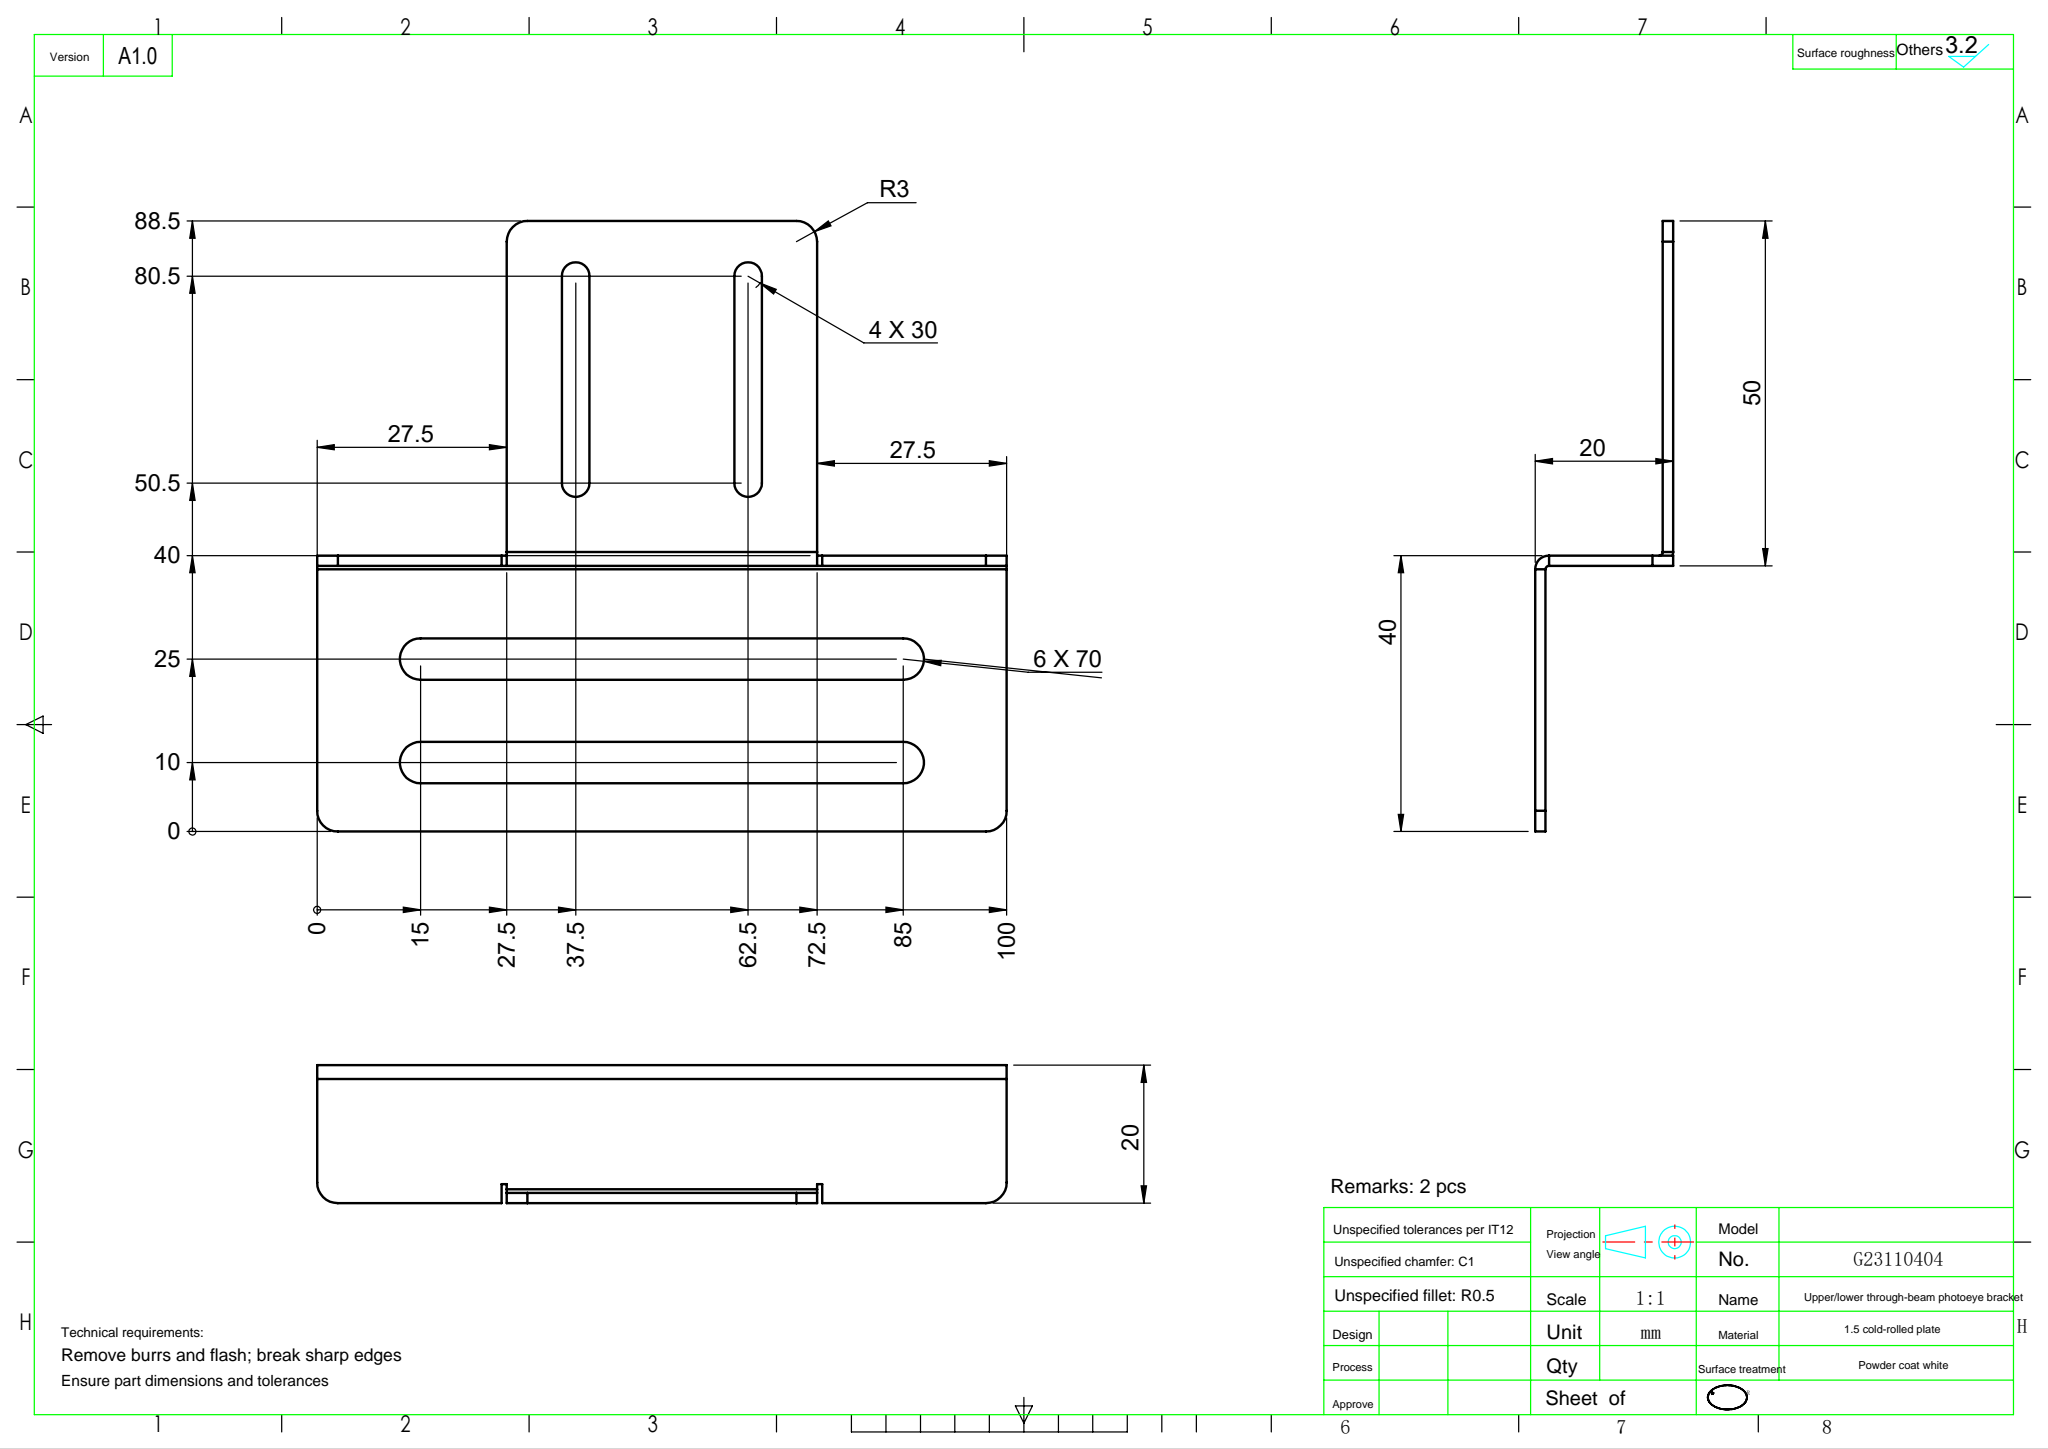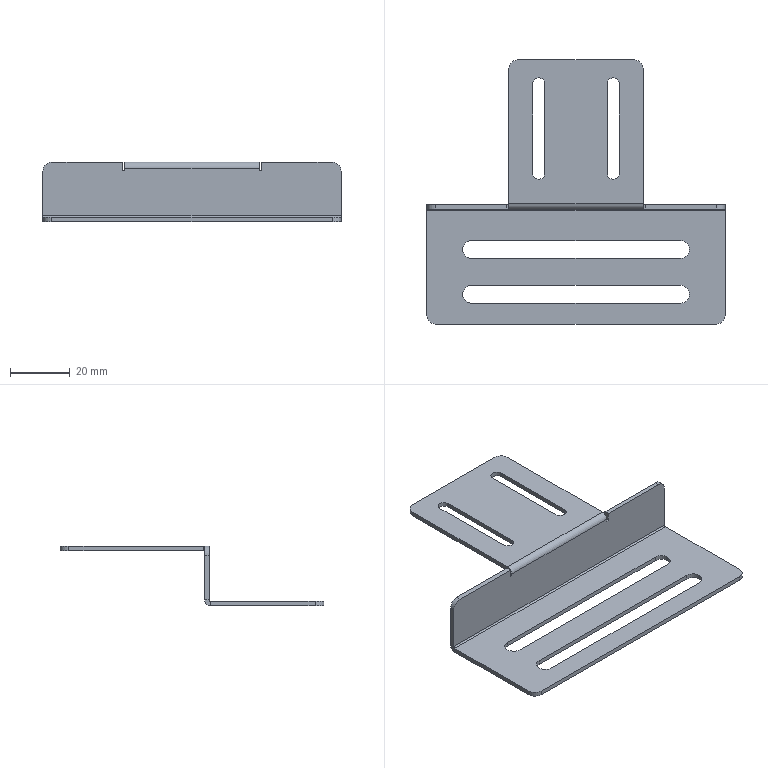Part | SolidWorks | features EdgeFlange 2, ICE 2, Fillet 1, FlatPattern 1, SMBaseFlange 1, SheetMetal 1 | 1 solid | 54 faces | box 100 x 88.5 x 20 mm | volume 10166 mm3 | plane 34 | cylinder 20 | commonest cylinder face diameters 6 x12 4 x6 1 x2